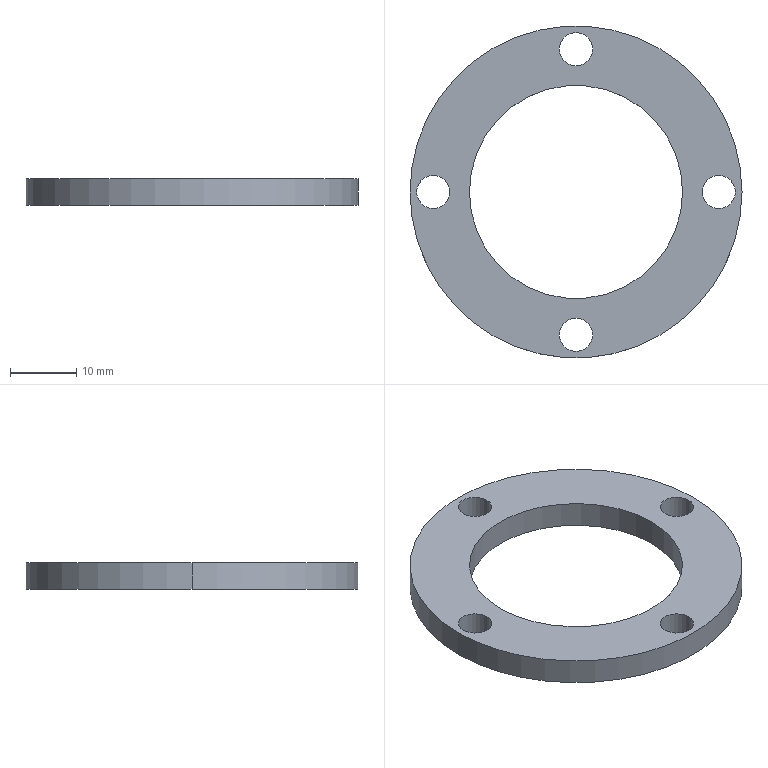Part | STEP file | X77-09004 | 1 solid | 14 faces | box 50 x 50 x 4 mm | volume 4303 mm3 | cylinder 12 | plane 2 | commonest cylinder face diameters 5 x8 32.1 x2 50 x2
STEP:
#1=CARTESIAN_POINT('',(200.447,151.671,4.));
#2=VERTEX_POINT('',#1);
#3=CARTESIAN_POINT('',(205.447,151.671,4.));
#4=VERTEX_POINT('',#3);
#5=CARTESIAN_POINT('',(202.947,151.671,4.));
#6=DIRECTION('',(0.,0.,1.));
#7=DIRECTION('',(1.,0.,0.));
#8=AXIS2_PLACEMENT_3D('',#5,#6,#7);
#9=CIRCLE('',#8,2.5);
#10=EDGE_CURVE('',#2,#4,#9,.T.);
#11=ORIENTED_EDGE('',*,*,#10,.T.);
#12=CARTESIAN_POINT('',(205.447,151.671,0.));
#13=VERTEX_POINT('',#12);
#14=CARTESIAN_POINT('',(205.447,151.671,4.));
#15=DIRECTION('',(0.,0.,-1.));
#16=VECTOR('',#15,1000.);
#17=LINE('',#14,#16);
#18=EDGE_CURVE('',#4,#13,#17,.T.);
#19=ORIENTED_EDGE('',*,*,#18,.T.);
#20=CARTESIAN_POINT('',(200.447,151.671,0.));
#21=VERTEX_POINT('',#20);
#22=CARTESIAN_POINT('',(202.947,151.671,0.));
#23=DIRECTION('',(0.,0.,1.));
#24=DIRECTION('',(1.,0.,0.));
#25=AXIS2_PLACEMENT_3D('',#22,#23,#24);
#26=CIRCLE('',#25,2.5);
#27=EDGE_CURVE('',#21,#13,#26,.T.);
#28=ORIENTED_EDGE('',*,*,#27,.F.);
#29=CARTESIAN_POINT('',(200.447,151.671,4.));
#30=DIRECTION('',(0.,0.,-1.));
#31=VECTOR('',#30,1000.);
#32=LINE('',#29,#31);
#33=EDGE_CURVE('',#2,#21,#32,.T.);
#34=ORIENTED_EDGE('',*,*,#33,.F.);
#35=EDGE_LOOP('',(#11,#19,#28,#34));
#36=FACE_OUTER_BOUND('',#35,.T.);
#37=CARTESIAN_POINT('',(202.947,151.671,4.));
#38=DIRECTION('',(0.,0.,-1.));
#39=DIRECTION('',(-1.,0.,0.));
#40=AXIS2_PLACEMENT_3D('',#37,#38,#39);
#41=CYLINDRICAL_SURFACE('',#40,2.5);
#42=ADVANCED_FACE('',(#36),#41,.F.);
#43=CARTESIAN_POINT('',(221.947,130.171,4.));
#44=VERTEX_POINT('',#43);
#45=CARTESIAN_POINT('',(226.947,130.171,4.));
#46=VERTEX_POINT('',#45);
#47=CARTESIAN_POINT('',(224.447,130.171,4.));
#48=DIRECTION('',(0.,0.,1.));
#49=DIRECTION('',(1.,0.,0.));
#50=AXIS2_PLACEMENT_3D('',#47,#48,#49);
#51=CIRCLE('',#50,2.5);
#52=EDGE_CURVE('',#44,#46,#51,.T.);
#53=ORIENTED_EDGE('',*,*,#52,.T.);
#54=CARTESIAN_POINT('',(226.947,130.171,0.));
#55=VERTEX_POINT('',#54);
#56=CARTESIAN_POINT('',(226.947,130.171,4.));
#57=DIRECTION('',(0.,0.,-1.));
#58=VECTOR('',#57,1000.);
#59=LINE('',#56,#58);
#60=EDGE_CURVE('',#46,#55,#59,.T.);
#61=ORIENTED_EDGE('',*,*,#60,.T.);
#62=CARTESIAN_POINT('',(221.947,130.171,0.));
#63=VERTEX_POINT('',#62);
#64=CARTESIAN_POINT('',(224.447,130.171,0.));
#65=DIRECTION('',(0.,0.,1.));
#66=DIRECTION('',(1.,0.,0.));
#67=AXIS2_PLACEMENT_3D('',#64,#65,#66);
#68=CIRCLE('',#67,2.5);
#69=EDGE_CURVE('',#63,#55,#68,.T.);
#70=ORIENTED_EDGE('',*,*,#69,.F.);
#71=CARTESIAN_POINT('',(221.947,130.171,4.));
#72=DIRECTION('',(0.,0.,-1.));
#73=VECTOR('',#72,1000.);
#74=LINE('',#71,#73);
#75=EDGE_CURVE('',#44,#63,#74,.T.);
#76=ORIENTED_EDGE('',*,*,#75,.F.);
#77=EDGE_LOOP('',(#53,#61,#70,#76));
#78=FACE_OUTER_BOUND('',#77,.T.);
#79=CARTESIAN_POINT('',(224.447,130.171,4.));
#80=DIRECTION('',(0.,0.,-1.));
#81=DIRECTION('',(-1.,0.,0.));
#82=AXIS2_PLACEMENT_3D('',#79,#80,#81);
#83=CYLINDRICAL_SURFACE('',#82,2.5);
#84=ADVANCED_FACE('',(#78),#83,.F.);
#85=CARTESIAN_POINT('',(243.447,151.671,4.));
#86=VERTEX_POINT('',#85);
#87=CARTESIAN_POINT('',(248.447,151.671,4.));
#88=VERTEX_POINT('',#87);
#89=CARTESIAN_POINT('',(245.947,151.671,4.));
#90=DIRECTION('',(0.,0.,1.));
#91=DIRECTION('',(1.,0.,0.));
#92=AXIS2_PLACEMENT_3D('',#89,#90,#91);
#93=CIRCLE('',#92,2.5);
#94=EDGE_CURVE('',#86,#88,#93,.T.);
#95=ORIENTED_EDGE('',*,*,#94,.T.);
#96=CARTESIAN_POINT('',(248.447,151.671,0.));
#97=VERTEX_POINT('',#96);
#98=CARTESIAN_POINT('',(248.447,151.671,4.));
#99=DIRECTION('',(0.,0.,-1.));
#100=VECTOR('',#99,1000.);
#101=LINE('',#98,#100);
#102=EDGE_CURVE('',#88,#97,#101,.T.);
#103=ORIENTED_EDGE('',*,*,#102,.T.);
#104=CARTESIAN_POINT('',(243.447,151.671,0.));
#105=VERTEX_POINT('',#104);
#106=CARTESIAN_POINT('',(245.947,151.671,0.));
#107=DIRECTION('',(0.,0.,1.));
#108=DIRECTION('',(1.,0.,0.));
#109=AXIS2_PLACEMENT_3D('',#106,#107,#108);
#110=CIRCLE('',#109,2.5);
#111=EDGE_CURVE('',#105,#97,#110,.T.);
#112=ORIENTED_EDGE('',*,*,#111,.F.);
#113=CARTESIAN_POINT('',(243.447,151.671,4.));
#114=DIRECTION('',(0.,0.,-1.));
#115=VECTOR('',#114,1000.);
#116=LINE('',#113,#115);
#117=EDGE_CURVE('',#86,#105,#116,.T.);
#118=ORIENTED_EDGE('',*,*,#117,.F.);
#119=EDGE_LOOP('',(#95,#103,#112,#118));
#120=FACE_OUTER_BOUND('',#119,.T.);
#121=CARTESIAN_POINT('',(245.947,151.671,4.));
#122=DIRECTION('',(0.,0.,-1.));
#123=DIRECTION('',(-1.,0.,0.));
#124=AXIS2_PLACEMENT_3D('',#121,#122,#123);
#125=CYLINDRICAL_SURFACE('',#124,2.5);
#126=ADVANCED_FACE('',(#120),#125,.F.);
#127=CARTESIAN_POINT('',(221.947,173.171,4.));
#128=VERTEX_POINT('',#127);
#129=CARTESIAN_POINT('',(226.947,173.171,4.));
#130=VERTEX_POINT('',#129);
#131=CARTESIAN_POINT('',(224.447,173.171,4.));
#132=DIRECTION('',(0.,0.,1.));
#133=DIRECTION('',(1.,0.,0.));
#134=AXIS2_PLACEMENT_3D('',#131,#132,#133);
#135=CIRCLE('',#134,2.5);
#136=EDGE_CURVE('',#128,#130,#135,.T.);
#137=ORIENTED_EDGE('',*,*,#136,.T.);
#138=CARTESIAN_POINT('',(226.947,173.171,0.));
#139=VERTEX_POINT('',#138);
#140=CARTESIAN_POINT('',(226.947,173.171,4.));
#141=DIRECTION('',(0.,0.,-1.));
#142=VECTOR('',#141,1000.);
#143=LINE('',#140,#142);
#144=EDGE_CURVE('',#130,#139,#143,.T.);
#145=ORIENTED_EDGE('',*,*,#144,.T.);
#146=CARTESIAN_POINT('',(221.947,173.171,0.));
#147=VERTEX_POINT('',#146);
#148=CARTESIAN_POINT('',(224.447,173.171,0.));
#149=DIRECTION('',(0.,0.,1.));
#150=DIRECTION('',(1.,0.,0.));
#151=AXIS2_PLACEMENT_3D('',#148,#149,#150);
#152=CIRCLE('',#151,2.5);
#153=EDGE_CURVE('',#147,#139,#152,.T.);
#154=ORIENTED_EDGE('',*,*,#153,.F.);
#155=CARTESIAN_POINT('',(221.947,173.171,4.));
#156=DIRECTION('',(0.,0.,-1.));
#157=VECTOR('',#156,1000.);
#158=LINE('',#155,#157);
#159=EDGE_CURVE('',#128,#147,#158,.T.);
#160=ORIENTED_EDGE('',*,*,#159,.F.);
#161=EDGE_LOOP('',(#137,#145,#154,#160));
#162=FACE_OUTER_BOUND('',#161,.T.);
#163=CARTESIAN_POINT('',(224.447,173.171,4.));
#164=DIRECTION('',(0.,0.,-1.));
#165=DIRECTION('',(-1.,0.,0.));
#166=AXIS2_PLACEMENT_3D('',#163,#164,#165);
#167=CYLINDRICAL_SURFACE('',#166,2.5);
#168=ADVANCED_FACE('',(#162),#167,.F.);
#169=CARTESIAN_POINT('',(208.397,151.671,4.));
#170=VERTEX_POINT('',#169);
#171=CARTESIAN_POINT('',(240.497,151.671,4.));
#172=VERTEX_POINT('',#171);
#173=CARTESIAN_POINT('',(224.447,151.671,4.));
#174=DIRECTION('',(0.,0.,1.));
#175=DIRECTION('',(1.,0.,0.));
#176=AXIS2_PLACEMENT_3D('',#173,#174,#175);
#177=CIRCLE('',#176,16.05);
#178=EDGE_CURVE('',#170,#172,#177,.T.);
#179=ORIENTED_EDGE('',*,*,#178,.T.);
#180=CARTESIAN_POINT('',(240.497,151.671,0.));
#181=VERTEX_POINT('',#180);
#182=CARTESIAN_POINT('',(240.497,151.671,4.));
#183=DIRECTION('',(0.,0.,-1.));
#184=VECTOR('',#183,1000.);
#185=LINE('',#182,#184);
#186=EDGE_CURVE('',#172,#181,#185,.T.);
#187=ORIENTED_EDGE('',*,*,#186,.T.);
#188=CARTESIAN_POINT('',(208.397,151.671,0.));
#189=VERTEX_POINT('',#188);
#190=CARTESIAN_POINT('',(224.447,151.671,0.));
#191=DIRECTION('',(0.,0.,1.));
#192=DIRECTION('',(1.,0.,0.));
#193=AXIS2_PLACEMENT_3D('',#190,#191,#192);
#194=CIRCLE('',#193,16.05);
#195=EDGE_CURVE('',#189,#181,#194,.T.);
#196=ORIENTED_EDGE('',*,*,#195,.F.);
#197=CARTESIAN_POINT('',(208.397,151.671,4.));
#198=DIRECTION('',(0.,0.,-1.));
#199=VECTOR('',#198,1000.);
#200=LINE('',#197,#199);
#201=EDGE_CURVE('',#170,#189,#200,.T.);
#202=ORIENTED_EDGE('',*,*,#201,.F.);
#203=EDGE_LOOP('',(#179,#187,#196,#202));
#204=FACE_OUTER_BOUND('',#203,.T.);
#205=CARTESIAN_POINT('',(224.447,151.671,4.));
#206=DIRECTION('',(0.,0.,-1.));
#207=DIRECTION('',(-1.,0.,0.));
#208=AXIS2_PLACEMENT_3D('',#205,#206,#207);
#209=CYLINDRICAL_SURFACE('',#208,16.05);
#210=ADVANCED_FACE('',(#204),#209,.F.);
#211=CARTESIAN_POINT('',(249.447,151.671,4.));
#212=VERTEX_POINT('',#211);
#213=CARTESIAN_POINT('',(199.447,151.671,4.));
#214=VERTEX_POINT('',#213);
#215=CARTESIAN_POINT('',(224.447,151.671,4.));
#216=DIRECTION('',(0.,0.,1.));
#217=DIRECTION('',(1.,0.,0.));
#218=AXIS2_PLACEMENT_3D('',#215,#216,#217);
#219=CIRCLE('',#218,25.);
#220=EDGE_CURVE('',#212,#214,#219,.T.);
#221=ORIENTED_EDGE('',*,*,#220,.F.);
#222=CARTESIAN_POINT('',(249.447,151.671,0.));
#223=VERTEX_POINT('',#222);
#224=CARTESIAN_POINT('',(249.447,151.671,4.));
#225=DIRECTION('',(0.,0.,-1.));
#226=VECTOR('',#225,1000.);
#227=LINE('',#224,#226);
#228=EDGE_CURVE('',#212,#223,#227,.T.);
#229=ORIENTED_EDGE('',*,*,#228,.T.);
#230=CARTESIAN_POINT('',(199.447,151.671,0.));
#231=VERTEX_POINT('',#230);
#232=CARTESIAN_POINT('',(224.447,151.671,0.));
#233=DIRECTION('',(0.,0.,1.));
#234=DIRECTION('',(1.,0.,0.));
#235=AXIS2_PLACEMENT_3D('',#232,#233,#234);
#236=CIRCLE('',#235,25.);
#237=EDGE_CURVE('',#223,#231,#236,.T.);
#238=ORIENTED_EDGE('',*,*,#237,.T.);
#239=CARTESIAN_POINT('',(199.447,151.671,4.));
#240=DIRECTION('',(0.,0.,-1.));
#241=VECTOR('',#240,1000.);
#242=LINE('',#239,#241);
#243=EDGE_CURVE('',#214,#231,#242,.T.);
#244=ORIENTED_EDGE('',*,*,#243,.F.);
#245=EDGE_LOOP('',(#221,#229,#238,#244));
#246=FACE_OUTER_BOUND('',#245,.T.);
#247=CARTESIAN_POINT('',(224.447,151.671,4.));
#248=DIRECTION('',(0.,0.,-1.));
#249=DIRECTION('',(-1.,0.,0.));
#250=AXIS2_PLACEMENT_3D('',#247,#248,#249);
#251=CYLINDRICAL_SURFACE('',#250,25.);
#252=ADVANCED_FACE('',(#246),#251,.T.);
#253=ORIENTED_EDGE('',*,*,#52,.F.);
#254=CARTESIAN_POINT('',(224.447,130.171,4.));
#255=DIRECTION('',(0.,0.,1.));
#256=DIRECTION('',(1.,0.,0.));
#257=AXIS2_PLACEMENT_3D('',#254,#255,#256);
#258=CIRCLE('',#257,2.5);
#259=EDGE_CURVE('',#46,#44,#258,.T.);
#260=ORIENTED_EDGE('',*,*,#259,.F.);
#261=EDGE_LOOP('',(#253,#260));
#262=FACE_BOUND('',#261,.T.);
#263=ORIENTED_EDGE('',*,*,#136,.F.);
#264=CARTESIAN_POINT('',(224.447,173.171,4.));
#265=DIRECTION('',(0.,0.,1.));
#266=DIRECTION('',(1.,0.,0.));
#267=AXIS2_PLACEMENT_3D('',#264,#265,#266);
#268=CIRCLE('',#267,2.5);
#269=EDGE_CURVE('',#130,#128,#268,.T.);
#270=ORIENTED_EDGE('',*,*,#269,.F.);
#271=EDGE_LOOP('',(#263,#270));
#272=FACE_BOUND('',#271,.T.);
#273=CARTESIAN_POINT('',(224.447,151.671,4.));
#274=DIRECTION('',(0.,0.,1.));
#275=DIRECTION('',(1.,0.,0.));
#276=AXIS2_PLACEMENT_3D('',#273,#274,#275);
#277=CIRCLE('',#276,25.);
#278=EDGE_CURVE('',#214,#212,#277,.T.);
#279=ORIENTED_EDGE('',*,*,#278,.T.);
#280=ORIENTED_EDGE('',*,*,#220,.T.);
#281=EDGE_LOOP('',(#279,#280));
#282=FACE_OUTER_BOUND('',#281,.T.);
#283=ORIENTED_EDGE('',*,*,#178,.F.);
#284=CARTESIAN_POINT('',(224.447,151.671,4.));
#285=DIRECTION('',(0.,0.,1.));
#286=DIRECTION('',(1.,0.,0.));
#287=AXIS2_PLACEMENT_3D('',#284,#285,#286);
#288=CIRCLE('',#287,16.05);
#289=EDGE_CURVE('',#172,#170,#288,.T.);
#290=ORIENTED_EDGE('',*,*,#289,.F.);
#291=EDGE_LOOP('',(#283,#290));
#292=FACE_BOUND('',#291,.T.);
#293=ORIENTED_EDGE('',*,*,#94,.F.);
#294=CARTESIAN_POINT('',(245.947,151.671,4.));
#295=DIRECTION('',(0.,0.,1.));
#296=DIRECTION('',(1.,0.,0.));
#297=AXIS2_PLACEMENT_3D('',#294,#295,#296);
#298=CIRCLE('',#297,2.5);
#299=EDGE_CURVE('',#88,#86,#298,.T.);
#300=ORIENTED_EDGE('',*,*,#299,.F.);
#301=EDGE_LOOP('',(#293,#300));
#302=FACE_BOUND('',#301,.T.);
#303=ORIENTED_EDGE('',*,*,#10,.F.);
#304=CARTESIAN_POINT('',(202.947,151.671,4.));
#305=DIRECTION('',(0.,0.,1.));
#306=DIRECTION('',(1.,0.,0.));
#307=AXIS2_PLACEMENT_3D('',#304,#305,#306);
#308=CIRCLE('',#307,2.5);
#309=EDGE_CURVE('',#4,#2,#308,.T.);
#310=ORIENTED_EDGE('',*,*,#309,.F.);
#311=EDGE_LOOP('',(#303,#310));
#312=FACE_BOUND('',#311,.T.);
#313=CARTESIAN_POINT('',(224.447,151.671,4.));
#314=DIRECTION('',(0.,0.,1.));
#315=DIRECTION('',(1.,0.,0.));
#316=AXIS2_PLACEMENT_3D('',#313,#314,#315);
#317=PLANE('',#316);
#318=ADVANCED_FACE('',(#262,#272,#282,#292,#302,#312),#317,.T.);
#319=ORIENTED_EDGE('',*,*,#69,.T.);
#320=CARTESIAN_POINT('',(224.447,130.171,0.));
#321=DIRECTION('',(0.,0.,1.));
#322=DIRECTION('',(1.,0.,0.));
#323=AXIS2_PLACEMENT_3D('',#320,#321,#322);
#324=CIRCLE('',#323,2.5);
#325=EDGE_CURVE('',#55,#63,#324,.T.);
#326=ORIENTED_EDGE('',*,*,#325,.T.);
#327=EDGE_LOOP('',(#319,#326));
#328=FACE_BOUND('',#327,.T.);
#329=ORIENTED_EDGE('',*,*,#153,.T.);
#330=CARTESIAN_POINT('',(224.447,173.171,0.));
#331=DIRECTION('',(0.,0.,1.));
#332=DIRECTION('',(1.,0.,0.));
#333=AXIS2_PLACEMENT_3D('',#330,#331,#332);
#334=CIRCLE('',#333,2.5);
#335=EDGE_CURVE('',#139,#147,#334,.T.);
#336=ORIENTED_EDGE('',*,*,#335,.T.);
#337=EDGE_LOOP('',(#329,#336));
#338=FACE_BOUND('',#337,.T.);
#339=CARTESIAN_POINT('',(224.447,151.671,0.));
#340=DIRECTION('',(0.,0.,1.));
#341=DIRECTION('',(1.,0.,0.));
#342=AXIS2_PLACEMENT_3D('',#339,#340,#341);
#343=CIRCLE('',#342,25.);
#344=EDGE_CURVE('',#231,#223,#343,.T.);
#345=ORIENTED_EDGE('',*,*,#344,.F.);
#346=ORIENTED_EDGE('',*,*,#237,.F.);
#347=EDGE_LOOP('',(#345,#346));
#348=FACE_OUTER_BOUND('',#347,.T.);
#349=ORIENTED_EDGE('',*,*,#195,.T.);
#350=CARTESIAN_POINT('',(224.447,151.671,0.));
#351=DIRECTION('',(0.,0.,1.));
#352=DIRECTION('',(1.,0.,0.));
#353=AXIS2_PLACEMENT_3D('',#350,#351,#352);
#354=CIRCLE('',#353,16.05);
#355=EDGE_CURVE('',#181,#189,#354,.T.);
#356=ORIENTED_EDGE('',*,*,#355,.T.);
#357=EDGE_LOOP('',(#349,#356));
#358=FACE_BOUND('',#357,.T.);
#359=ORIENTED_EDGE('',*,*,#111,.T.);
#360=CARTESIAN_POINT('',(245.947,151.671,0.));
#361=DIRECTION('',(0.,0.,1.));
#362=DIRECTION('',(1.,0.,0.));
#363=AXIS2_PLACEMENT_3D('',#360,#361,#362);
#364=CIRCLE('',#363,2.5);
#365=EDGE_CURVE('',#97,#105,#364,.T.);
#366=ORIENTED_EDGE('',*,*,#365,.T.);
#367=EDGE_LOOP('',(#359,#366));
#368=FACE_BOUND('',#367,.T.);
#369=ORIENTED_EDGE('',*,*,#27,.T.);
#370=CARTESIAN_POINT('',(202.947,151.671,0.));
#371=DIRECTION('',(0.,0.,1.));
#372=DIRECTION('',(1.,0.,0.));
#373=AXIS2_PLACEMENT_3D('',#370,#371,#372);
#374=CIRCLE('',#373,2.5);
#375=EDGE_CURVE('',#13,#21,#374,.T.);
#376=ORIENTED_EDGE('',*,*,#375,.T.);
#377=EDGE_LOOP('',(#369,#376));
#378=FACE_BOUND('',#377,.T.);
#379=CARTESIAN_POINT('',(224.447,151.671,0.));
#380=DIRECTION('',(0.,0.,1.));
#381=DIRECTION('',(1.,0.,0.));
#382=AXIS2_PLACEMENT_3D('',#379,#380,#381);
#383=PLANE('',#382);
#384=ADVANCED_FACE('',(#328,#338,#348,#358,#368,#378),#383,.F.);
#385=ORIENTED_EDGE('',*,*,#228,.F.);
#386=ORIENTED_EDGE('',*,*,#278,.F.);
#387=ORIENTED_EDGE('',*,*,#243,.T.);
#388=ORIENTED_EDGE('',*,*,#344,.T.);
#389=EDGE_LOOP('',(#385,#386,#387,#388));
#390=FACE_OUTER_BOUND('',#389,.T.);
#391=CARTESIAN_POINT('',(224.447,151.671,4.));
#392=DIRECTION('',(0.,0.,-1.));
#393=DIRECTION('',(-1.,0.,0.));
#394=AXIS2_PLACEMENT_3D('',#391,#392,#393);
#395=CYLINDRICAL_SURFACE('',#394,25.);
#396=ADVANCED_FACE('',(#390),#395,.T.);
#397=ORIENTED_EDGE('',*,*,#186,.F.);
#398=ORIENTED_EDGE('',*,*,#289,.T.);
#399=ORIENTED_EDGE('',*,*,#201,.T.);
#400=ORIENTED_EDGE('',*,*,#355,.F.);
#401=EDGE_LOOP('',(#397,#398,#399,#400));
#402=FACE_OUTER_BOUND('',#401,.T.);
#403=CARTESIAN_POINT('',(224.447,151.671,4.));
#404=DIRECTION('',(0.,0.,-1.));
#405=DIRECTION('',(-1.,0.,0.));
#406=AXIS2_PLACEMENT_3D('',#403,#404,#405);
#407=CYLINDRICAL_SURFACE('',#406,16.05);
#408=ADVANCED_FACE('',(#402),#407,.F.);
#409=ORIENTED_EDGE('',*,*,#144,.F.);
#410=ORIENTED_EDGE('',*,*,#269,.T.);
#411=ORIENTED_EDGE('',*,*,#159,.T.);
#412=ORIENTED_EDGE('',*,*,#335,.F.);
#413=EDGE_LOOP('',(#409,#410,#411,#412));
#414=FACE_OUTER_BOUND('',#413,.T.);
#415=CARTESIAN_POINT('',(224.447,173.171,4.));
#416=DIRECTION('',(0.,0.,-1.));
#417=DIRECTION('',(-1.,0.,0.));
#418=AXIS2_PLACEMENT_3D('',#415,#416,#417);
#419=CYLINDRICAL_SURFACE('',#418,2.5);
#420=ADVANCED_FACE('',(#414),#419,.F.);
#421=ORIENTED_EDGE('',*,*,#102,.F.);
#422=ORIENTED_EDGE('',*,*,#299,.T.);
#423=ORIENTED_EDGE('',*,*,#117,.T.);
#424=ORIENTED_EDGE('',*,*,#365,.F.);
#425=EDGE_LOOP('',(#421,#422,#423,#424));
#426=FACE_OUTER_BOUND('',#425,.T.);
#427=CARTESIAN_POINT('',(245.947,151.671,4.));
#428=DIRECTION('',(0.,0.,-1.));
#429=DIRECTION('',(-1.,0.,0.));
#430=AXIS2_PLACEMENT_3D('',#427,#428,#429);
#431=CYLINDRICAL_SURFACE('',#430,2.5);
#432=ADVANCED_FACE('',(#426),#431,.F.);
#433=ORIENTED_EDGE('',*,*,#60,.F.);
#434=ORIENTED_EDGE('',*,*,#259,.T.);
#435=ORIENTED_EDGE('',*,*,#75,.T.);
#436=ORIENTED_EDGE('',*,*,#325,.F.);
#437=EDGE_LOOP('',(#433,#434,#435,#436));
#438=FACE_OUTER_BOUND('',#437,.T.);
#439=CARTESIAN_POINT('',(224.447,130.171,4.));
#440=DIRECTION('',(0.,0.,-1.));
#441=DIRECTION('',(-1.,0.,0.));
#442=AXIS2_PLACEMENT_3D('',#439,#440,#441);
#443=CYLINDRICAL_SURFACE('',#442,2.5);
#444=ADVANCED_FACE('',(#438),#443,.F.);
#445=ORIENTED_EDGE('',*,*,#18,.F.);
#446=ORIENTED_EDGE('',*,*,#309,.T.);
#447=ORIENTED_EDGE('',*,*,#33,.T.);
#448=ORIENTED_EDGE('',*,*,#375,.F.);
#449=EDGE_LOOP('',(#445,#446,#447,#448));
#450=FACE_OUTER_BOUND('',#449,.T.);
#451=CARTESIAN_POINT('',(202.947,151.671,4.));
#452=DIRECTION('',(0.,0.,-1.));
#453=DIRECTION('',(-1.,0.,0.));
#454=AXIS2_PLACEMENT_3D('',#451,#452,#453);
#455=CYLINDRICAL_SURFACE('',#454,2.5);
#456=ADVANCED_FACE('',(#450),#455,.F.);
#457=CLOSED_SHELL('',(#42,#84,#126,#168,#210,#252,#318,#384,#396,#408,#420,#432,#444,#456));
#458=MANIFOLD_SOLID_BREP('',#457);
#459=CARTESIAN_POINT('',(0.,0.,0.));
#460=DIRECTION('',(0.,0.,1.));
#461=DIRECTION('',(1.,0.,0.));
#462=AXIS2_PLACEMENT_3D('',#459,#460,#461);
#463=(LENGTH_UNIT()NAMED_UNIT(*)SI_UNIT(.MILLI.,.METRE.));
#464=UNCERTAINTY_MEASURE_WITH_UNIT(LENGTH_MEASURE(0.00001),#463,'','');
#465=(NAMED_UNIT(*)PLANE_ANGLE_UNIT()SI_UNIT($,.RADIAN.));
#466=(NAMED_UNIT(*)SI_UNIT($,.STERADIAN.)SOLID_ANGLE_UNIT());
#467=(GEOMETRIC_REPRESENTATION_CONTEXT(3)GLOBAL_UNCERTAINTY_ASSIGNED_CONTEXT((#464))GLOBAL_UNIT_ASSIGNED_CONTEXT((#463,#465,#466))REPRESENTATION_CONTEXT('',''));
#468=ADVANCED_BREP_SHAPE_REPRESENTATION('',(#458,#462),#467);